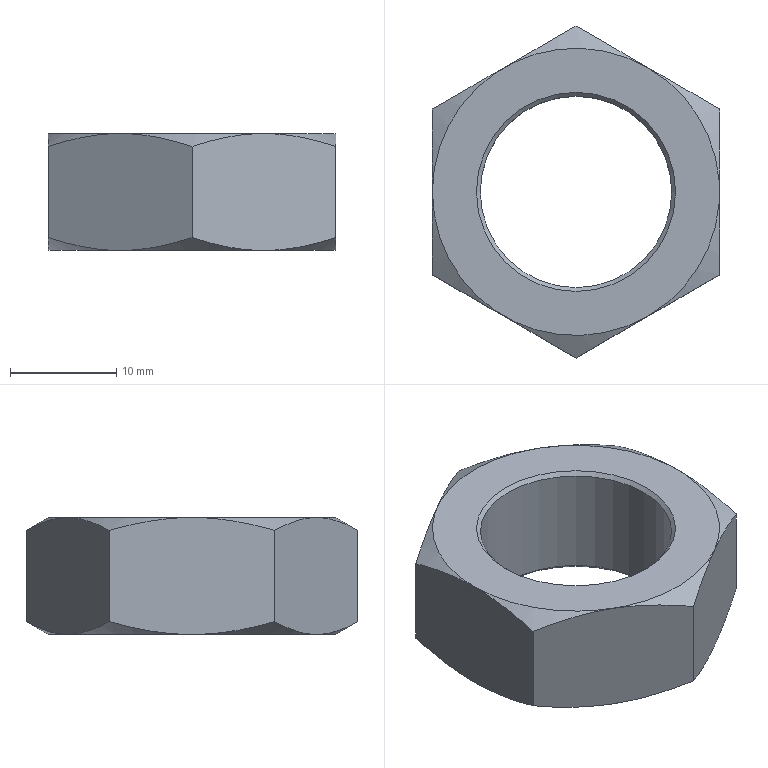Part | NX | features Hydraulic2.3_M18X1.5 2 | 1 solid | 13 faces | box 27.02 x 31.2 x 11 mm | volume 4104 mm3 | plane 8 | cone 4 | cylinder 1 | commonest cylinder face diameters 18 x1
STEP:
#1=CARTESIAN_POINT('',(-13.5,0.,5.5));
#2=VERTEX_POINT('',#1);
#3=CARTESIAN_POINT('',(0.,0.,5.5));
#4=DIRECTION('',(0.,0.,-1.));
#5=DIRECTION('',(-1.,0.,0.));
#6=AXIS2_PLACEMENT_3D('',#3,#4,#5);
#7=CIRCLE('',#6,13.5);
#8=EDGE_CURVE('',#2,#2,#7,.T.);
#9=ORIENTED_EDGE('',*,*,#8,.F.);
#10=EDGE_LOOP('',(#9));
#11=FACE_BOUND('',#10,.T.);
#12=CARTESIAN_POINT('',(9.36,0.,5.5));
#13=VERTEX_POINT('',#12);
#14=CARTESIAN_POINT('',(0.,0.,5.5));
#15=DIRECTION('',(0.,0.,1.));
#16=DIRECTION('',(1.,0.,0.));
#17=AXIS2_PLACEMENT_3D('',#14,#15,#16);
#18=CIRCLE('',#17,9.36);
#19=EDGE_CURVE('',#13,#13,#18,.F.);
#20=ORIENTED_EDGE('',*,*,#19,.T.);
#21=EDGE_LOOP('',(#20));
#22=FACE_BOUND('',#21,.T.);
#23=CARTESIAN_POINT('',(0.,9.,5.5));
#24=DIRECTION('',(0.,0.,1.));
#25=DIRECTION('',(0.,-1.,0.));
#26=AXIS2_PLACEMENT_3D('',#23,#24,#25);
#27=PLANE('',#26);
#28=ADVANCED_FACE('',(#11,#22),#27,.T.);
#29=CARTESIAN_POINT('',(0.,9.,5.14));
#30=VERTEX_POINT('',#29);
#31=CARTESIAN_POINT('',(0.,0.,5.14));
#32=DIRECTION('',(0.,0.,-1.));
#33=DIRECTION('',(0.,1.,0.));
#34=AXIS2_PLACEMENT_3D('',#31,#32,#33);
#35=CIRCLE('',#34,9.);
#36=EDGE_CURVE('',#30,#30,#35,.T.);
#37=ORIENTED_EDGE('',*,*,#36,.T.);
#38=EDGE_LOOP('',(#37));
#39=FACE_BOUND('',#38,.T.);
#40=ORIENTED_EDGE('',*,*,#19,.F.);
#41=EDGE_LOOP('',(#40));
#42=FACE_BOUND('',#41,.T.);
#43=CARTESIAN_POINT('',(0.,0.,5.5));
#44=DIRECTION('',(0.,0.,1.));
#45=DIRECTION('',(1.,0.,0.));
#46=AXIS2_PLACEMENT_3D('',#43,#44,#45);
#47=CONICAL_SURFACE('',#46,9.36,0.7854);
#48=ADVANCED_FACE('',(#39,#42),#47,.F.);
#49=ORIENTED_EDGE('',*,*,#8,.T.);
#50=EDGE_LOOP('',(#49));
#51=FACE_BOUND('',#50,.T.);
#52=CARTESIAN_POINT('',(13.51,-7.8,4.288));
#53=VERTEX_POINT('',#52);
#54=CARTESIAN_POINT('',(0.,-15.6,4.288));
#55=VERTEX_POINT('',#54);
#56=CARTESIAN_POINT('',(13.51,-7.8,4.288));
#57=CARTESIAN_POINT('',(11.304,-9.074,5.023));
#58=CARTESIAN_POINT('',(6.779,-11.686,5.965));
#59=CARTESIAN_POINT('',(2.209,-14.325,5.024));
#60=CARTESIAN_POINT('',(0.,-15.6,4.288));
#61=B_SPLINE_CURVE_WITH_KNOTS('',3,(#56,#57,#58,#59,#60),.UNSPECIFIED.,.F.,.F.,(4,1,4),(0.,0.007878,0.01576),.UNSPECIFIED.);
#62=EDGE_CURVE('',#53,#55,#61,.T.);
#63=ORIENTED_EDGE('',*,*,#62,.F.);
#64=CARTESIAN_POINT('',(13.51,7.8,4.288));
#65=VERTEX_POINT('',#64);
#66=CARTESIAN_POINT('',(13.51,7.8,4.288));
#67=CARTESIAN_POINT('',(13.51,5.252,5.023));
#68=CARTESIAN_POINT('',(13.51,0.,5.965));
#69=CARTESIAN_POINT('',(13.51,-5.252,5.023));
#70=CARTESIAN_POINT('',(13.51,-7.8,4.288));
#71=B_SPLINE_CURVE_WITH_KNOTS('',3,(#66,#67,#68,#69,#70),.UNSPECIFIED.,.F.,.F.,(4,1,4),(-0.007893,0.,0.007893),.UNSPECIFIED.);
#72=EDGE_CURVE('',#65,#53,#71,.T.);
#73=ORIENTED_EDGE('',*,*,#72,.F.);
#74=CARTESIAN_POINT('',(0.,15.6,4.288));
#75=VERTEX_POINT('',#74);
#76=CARTESIAN_POINT('',(0.,15.6,4.288));
#77=CARTESIAN_POINT('',(2.206,14.326,5.023));
#78=CARTESIAN_POINT('',(6.731,11.714,5.965));
#79=CARTESIAN_POINT('',(11.301,9.075,5.024));
#80=CARTESIAN_POINT('',(13.51,7.8,4.288));
#81=B_SPLINE_CURVE_WITH_KNOTS('',3,(#76,#77,#78,#79,#80),.UNSPECIFIED.,.F.,.F.,(4,1,4),(0.,0.007878,0.01576),.UNSPECIFIED.);
#82=EDGE_CURVE('',#75,#65,#81,.T.);
#83=ORIENTED_EDGE('',*,*,#82,.F.);
#84=CARTESIAN_POINT('',(-13.51,7.8,4.288));
#85=VERTEX_POINT('',#84);
#86=CARTESIAN_POINT('',(-13.51,7.8,4.288));
#87=CARTESIAN_POINT('',(-11.304,9.074,5.023));
#88=CARTESIAN_POINT('',(-6.779,11.686,5.965));
#89=CARTESIAN_POINT('',(-2.209,14.325,5.024));
#90=CARTESIAN_POINT('',(0.,15.6,4.288));
#91=B_SPLINE_CURVE_WITH_KNOTS('',3,(#86,#87,#88,#89,#90),.UNSPECIFIED.,.F.,.F.,(4,1,4),(0.,0.007878,0.01576),.UNSPECIFIED.);
#92=EDGE_CURVE('',#85,#75,#91,.T.);
#93=ORIENTED_EDGE('',*,*,#92,.F.);
#94=CARTESIAN_POINT('',(-13.51,-7.8,4.288));
#95=VERTEX_POINT('',#94);
#96=CARTESIAN_POINT('',(-13.51,-7.8,4.288));
#97=CARTESIAN_POINT('',(-13.51,-5.252,5.023));
#98=CARTESIAN_POINT('',(-13.51,0.,5.965));
#99=CARTESIAN_POINT('',(-13.51,5.252,5.023));
#100=CARTESIAN_POINT('',(-13.51,7.8,4.288));
#101=B_SPLINE_CURVE_WITH_KNOTS('',3,(#96,#97,#98,#99,#100),.UNSPECIFIED.,.F.,.F.,(4,1,4),(-0.007893,0.,0.007893),.UNSPECIFIED.);
#102=EDGE_CURVE('',#95,#85,#101,.T.);
#103=ORIENTED_EDGE('',*,*,#102,.F.);
#104=CARTESIAN_POINT('',(0.,-15.6,4.288));
#105=CARTESIAN_POINT('',(-2.206,-14.326,5.023));
#106=CARTESIAN_POINT('',(-6.731,-11.714,5.965));
#107=CARTESIAN_POINT('',(-11.301,-9.075,5.024));
#108=CARTESIAN_POINT('',(-13.51,-7.8,4.288));
#109=B_SPLINE_CURVE_WITH_KNOTS('',3,(#104,#105,#106,#107,#108),.UNSPECIFIED.,.F.,.F.,(4,1,4),(0.,0.007878,0.01576),.UNSPECIFIED.);
#110=EDGE_CURVE('',#55,#95,#109,.T.);
#111=ORIENTED_EDGE('',*,*,#110,.F.);
#112=EDGE_LOOP('',(#63,#73,#83,#93,#103,#111));
#113=FACE_BOUND('',#112,.T.);
#114=CARTESIAN_POINT('',(0.,0.,4.28));
#115=DIRECTION('',(0.,0.,-1.));
#116=DIRECTION('',(-1.,0.,0.));
#117=AXIS2_PLACEMENT_3D('',#114,#115,#116);
#118=CONICAL_SURFACE('',#117,15.613,1.047);
#119=ADVANCED_FACE('',(#51,#113),#118,.T.);
#120=ORIENTED_EDGE('',*,*,#36,.F.);
#121=EDGE_LOOP('',(#120));
#122=FACE_BOUND('',#121,.T.);
#123=CARTESIAN_POINT('',(-9.,0.,-5.14));
#124=VERTEX_POINT('',#123);
#125=CARTESIAN_POINT('',(0.,0.,-5.14));
#126=DIRECTION('',(0.,0.,-1.));
#127=DIRECTION('',(-1.,0.,0.));
#128=AXIS2_PLACEMENT_3D('',#125,#126,#127);
#129=CIRCLE('',#128,9.);
#130=EDGE_CURVE('',#124,#124,#129,.T.);
#131=ORIENTED_EDGE('',*,*,#130,.T.);
#132=EDGE_LOOP('',(#131));
#133=FACE_BOUND('',#132,.T.);
#134=CARTESIAN_POINT('',(0.,0.,27.389));
#135=DIRECTION('',(0.,0.,-1.));
#136=DIRECTION('',(0.,1.,0.));
#137=AXIS2_PLACEMENT_3D('',#134,#135,#136);
#138=CYLINDRICAL_SURFACE('',#137,9.);
#139=ADVANCED_FACE('',(#122,#133),#138,.F.);
#140=CARTESIAN_POINT('',(0.000000014,-15.6,-4.288));
#141=VERTEX_POINT('',#140);
#142=CARTESIAN_POINT('',(0.,-15.6,-5.5));
#143=DIRECTION('',(0.,0.,1.));
#144=VECTOR('',#143,1000.);
#145=LINE('',#142,#144);
#146=EDGE_CURVE('',#141,#55,#145,.T.);
#147=ORIENTED_EDGE('',*,*,#146,.F.);
#148=CARTESIAN_POINT('',(13.51,-7.8,-4.288));
#149=VERTEX_POINT('',#148);
#150=CARTESIAN_POINT('',(13.51,-7.8,-4.288));
#151=CARTESIAN_POINT('',(11.304,-9.074,-5.023));
#152=CARTESIAN_POINT('',(6.779,-11.686,-5.965));
#153=CARTESIAN_POINT('',(2.209,-14.325,-5.024));
#154=CARTESIAN_POINT('',(0.000000075,-15.6,-4.288));
#155=B_SPLINE_CURVE_WITH_KNOTS('',3,(#150,#151,#152,#153,#154),.UNSPECIFIED.,.F.,.F.,(4,1,4),(0.,0.007878,0.01576),.UNSPECIFIED.);
#156=EDGE_CURVE('',#149,#141,#155,.T.);
#157=ORIENTED_EDGE('',*,*,#156,.F.);
#158=CARTESIAN_POINT('',(13.51,-7.8,-5.5));
#159=DIRECTION('',(0.,0.,1.));
#160=VECTOR('',#159,1000.);
#161=LINE('',#158,#160);
#162=EDGE_CURVE('',#53,#149,#161,.F.);
#163=ORIENTED_EDGE('',*,*,#162,.F.);
#164=ORIENTED_EDGE('',*,*,#62,.T.);
#165=EDGE_LOOP('',(#147,#157,#163,#164));
#166=FACE_BOUND('',#165,.T.);
#167=CARTESIAN_POINT('',(0.,-15.6,-5.5));
#168=DIRECTION('',(0.5,-0.866,0.));
#169=DIRECTION('',(0.866,0.5,0.));
#170=AXIS2_PLACEMENT_3D('',#167,#168,#169);
#171=PLANE('',#170);
#172=ADVANCED_FACE('',(#166),#171,.T.);
#173=CARTESIAN_POINT('',(-13.51,-7.8,-4.288));
#174=VERTEX_POINT('',#173);
#175=CARTESIAN_POINT('',(-13.51,-7.8,-5.5));
#176=DIRECTION('',(0.,0.,1.));
#177=VECTOR('',#176,1000.);
#178=LINE('',#175,#177);
#179=EDGE_CURVE('',#174,#95,#178,.T.);
#180=ORIENTED_EDGE('',*,*,#179,.F.);
#181=CARTESIAN_POINT('',(0.000000042,-15.6,-4.288));
#182=CARTESIAN_POINT('',(-2.206,-14.326,-5.023));
#183=CARTESIAN_POINT('',(-6.731,-11.714,-5.965));
#184=CARTESIAN_POINT('',(-11.301,-9.075,-5.024));
#185=CARTESIAN_POINT('',(-13.51,-7.8,-4.288));
#186=B_SPLINE_CURVE_WITH_KNOTS('',3,(#181,#182,#183,#184,#185),.UNSPECIFIED.,.F.,.F.,(4,1,4),(0.,0.007878,0.01576),.UNSPECIFIED.);
#187=EDGE_CURVE('',#141,#174,#186,.T.);
#188=ORIENTED_EDGE('',*,*,#187,.F.);
#189=ORIENTED_EDGE('',*,*,#146,.T.);
#190=ORIENTED_EDGE('',*,*,#110,.T.);
#191=EDGE_LOOP('',(#180,#188,#189,#190));
#192=FACE_BOUND('',#191,.T.);
#193=CARTESIAN_POINT('',(-13.51,-7.8,-5.5));
#194=DIRECTION('',(-0.5,-0.866,0.));
#195=DIRECTION('',(0.866,-0.5,0.));
#196=AXIS2_PLACEMENT_3D('',#193,#194,#195);
#197=PLANE('',#196);
#198=ADVANCED_FACE('',(#192),#197,.T.);
#199=CARTESIAN_POINT('',(-13.51,7.8,-4.288));
#200=VERTEX_POINT('',#199);
#201=CARTESIAN_POINT('',(-13.51,-7.8,-4.288));
#202=CARTESIAN_POINT('',(-13.51,-5.252,-5.023));
#203=CARTESIAN_POINT('',(-13.51,0.000000059,-5.965));
#204=CARTESIAN_POINT('',(-13.51,5.252,-5.023));
#205=CARTESIAN_POINT('',(-13.51,7.8,-4.288));
#206=B_SPLINE_CURVE_WITH_KNOTS('',3,(#201,#202,#203,#204,#205),.UNSPECIFIED.,.F.,.F.,(4,1,4),(-0.007893,0.,0.007893),.UNSPECIFIED.);
#207=EDGE_CURVE('',#174,#200,#206,.T.);
#208=ORIENTED_EDGE('',*,*,#207,.F.);
#209=ORIENTED_EDGE('',*,*,#179,.T.);
#210=ORIENTED_EDGE('',*,*,#102,.T.);
#211=CARTESIAN_POINT('',(-13.51,7.8,-5.5));
#212=DIRECTION('',(0.,0.,1.));
#213=VECTOR('',#212,1000.);
#214=LINE('',#211,#213);
#215=EDGE_CURVE('',#200,#85,#214,.T.);
#216=ORIENTED_EDGE('',*,*,#215,.F.);
#217=EDGE_LOOP('',(#208,#209,#210,#216));
#218=FACE_BOUND('',#217,.T.);
#219=CARTESIAN_POINT('',(-13.51,7.8,-5.5));
#220=DIRECTION('',(-1.,0.,0.));
#221=DIRECTION('',(0.,-1.,0.));
#222=AXIS2_PLACEMENT_3D('',#219,#220,#221);
#223=PLANE('',#222);
#224=ADVANCED_FACE('',(#218),#223,.T.);
#225=CARTESIAN_POINT('',(-0.000000014,15.6,-4.288));
#226=VERTEX_POINT('',#225);
#227=CARTESIAN_POINT('',(0.,15.6,-5.5));
#228=DIRECTION('',(0.,0.,1.));
#229=VECTOR('',#228,1000.);
#230=LINE('',#227,#229);
#231=EDGE_CURVE('',#226,#75,#230,.T.);
#232=ORIENTED_EDGE('',*,*,#231,.F.);
#233=CARTESIAN_POINT('',(-13.51,7.8,-4.288));
#234=CARTESIAN_POINT('',(-11.304,9.074,-5.023));
#235=CARTESIAN_POINT('',(-6.779,11.686,-5.965));
#236=CARTESIAN_POINT('',(-2.209,14.325,-5.024));
#237=CARTESIAN_POINT('',(-0.000000075,15.6,-4.288));
#238=B_SPLINE_CURVE_WITH_KNOTS('',3,(#233,#234,#235,#236,#237),.UNSPECIFIED.,.F.,.F.,(4,1,4),(0.,0.007878,0.01576),.UNSPECIFIED.);
#239=EDGE_CURVE('',#200,#226,#238,.T.);
#240=ORIENTED_EDGE('',*,*,#239,.F.);
#241=ORIENTED_EDGE('',*,*,#215,.T.);
#242=ORIENTED_EDGE('',*,*,#92,.T.);
#243=EDGE_LOOP('',(#232,#240,#241,#242));
#244=FACE_BOUND('',#243,.T.);
#245=CARTESIAN_POINT('',(0.,15.6,-5.5));
#246=DIRECTION('',(-0.5,0.866,0.));
#247=DIRECTION('',(-0.866,-0.5,0.));
#248=AXIS2_PLACEMENT_3D('',#245,#246,#247);
#249=PLANE('',#248);
#250=ADVANCED_FACE('',(#244),#249,.T.);
#251=CARTESIAN_POINT('',(13.51,7.8,-4.288));
#252=VERTEX_POINT('',#251);
#253=CARTESIAN_POINT('',(13.51,7.8,-5.5));
#254=DIRECTION('',(0.,0.,1.));
#255=VECTOR('',#254,1000.);
#256=LINE('',#253,#255);
#257=EDGE_CURVE('',#252,#65,#256,.T.);
#258=ORIENTED_EDGE('',*,*,#257,.F.);
#259=CARTESIAN_POINT('',(-0.000000029,15.6,-4.288));
#260=CARTESIAN_POINT('',(2.206,14.326,-5.023));
#261=CARTESIAN_POINT('',(6.731,11.714,-5.965));
#262=CARTESIAN_POINT('',(11.301,9.075,-5.024));
#263=CARTESIAN_POINT('',(13.51,7.8,-4.288));
#264=B_SPLINE_CURVE_WITH_KNOTS('',3,(#259,#260,#261,#262,#263),.UNSPECIFIED.,.F.,.F.,(4,1,4),(0.,0.007878,0.01576),.UNSPECIFIED.);
#265=EDGE_CURVE('',#226,#252,#264,.T.);
#266=ORIENTED_EDGE('',*,*,#265,.F.);
#267=ORIENTED_EDGE('',*,*,#231,.T.);
#268=ORIENTED_EDGE('',*,*,#82,.T.);
#269=EDGE_LOOP('',(#258,#266,#267,#268));
#270=FACE_BOUND('',#269,.T.);
#271=CARTESIAN_POINT('',(13.51,7.8,-5.5));
#272=DIRECTION('',(0.5,0.866,0.));
#273=DIRECTION('',(-0.866,0.5,0.));
#274=AXIS2_PLACEMENT_3D('',#271,#272,#273);
#275=PLANE('',#274);
#276=ADVANCED_FACE('',(#270),#275,.T.);
#277=ORIENTED_EDGE('',*,*,#162,.T.);
#278=CARTESIAN_POINT('',(13.51,7.8,-4.288));
#279=CARTESIAN_POINT('',(13.51,5.252,-5.023));
#280=CARTESIAN_POINT('',(13.51,-0.000000059,-5.965));
#281=CARTESIAN_POINT('',(13.51,-5.252,-5.023));
#282=CARTESIAN_POINT('',(13.51,-7.8,-4.288));
#283=B_SPLINE_CURVE_WITH_KNOTS('',3,(#278,#279,#280,#281,#282),.UNSPECIFIED.,.F.,.F.,(4,1,4),(0.,0.007893,0.01579),.UNSPECIFIED.);
#284=EDGE_CURVE('',#252,#149,#283,.T.);
#285=ORIENTED_EDGE('',*,*,#284,.F.);
#286=ORIENTED_EDGE('',*,*,#257,.T.);
#287=ORIENTED_EDGE('',*,*,#72,.T.);
#288=EDGE_LOOP('',(#277,#285,#286,#287));
#289=FACE_BOUND('',#288,.T.);
#290=CARTESIAN_POINT('',(13.51,-7.8,-5.5));
#291=DIRECTION('',(1.,0.,0.));
#292=DIRECTION('',(0.,1.,0.));
#293=AXIS2_PLACEMENT_3D('',#290,#291,#292);
#294=PLANE('',#293);
#295=ADVANCED_FACE('',(#289),#294,.T.);
#296=ORIENTED_EDGE('',*,*,#130,.F.);
#297=EDGE_LOOP('',(#296));
#298=FACE_BOUND('',#297,.T.);
#299=CARTESIAN_POINT('',(-9.36,0.,-5.5));
#300=VERTEX_POINT('',#299);
#301=CARTESIAN_POINT('',(0.,0.,-5.5));
#302=DIRECTION('',(0.,0.,-1.));
#303=DIRECTION('',(-1.,0.,0.));
#304=AXIS2_PLACEMENT_3D('',#301,#302,#303);
#305=CIRCLE('',#304,9.36);
#306=EDGE_CURVE('',#300,#300,#305,.F.);
#307=ORIENTED_EDGE('',*,*,#306,.F.);
#308=EDGE_LOOP('',(#307));
#309=FACE_BOUND('',#308,.T.);
#310=CARTESIAN_POINT('',(0.,0.,-5.5));
#311=DIRECTION('',(0.,0.,-1.));
#312=DIRECTION('',(-1.,0.,0.));
#313=AXIS2_PLACEMENT_3D('',#310,#311,#312);
#314=CONICAL_SURFACE('',#313,9.36,0.7854);
#315=ADVANCED_FACE('',(#298,#309),#314,.F.);
#316=ORIENTED_EDGE('',*,*,#187,.T.);
#317=ORIENTED_EDGE('',*,*,#207,.T.);
#318=ORIENTED_EDGE('',*,*,#239,.T.);
#319=ORIENTED_EDGE('',*,*,#265,.T.);
#320=ORIENTED_EDGE('',*,*,#284,.T.);
#321=ORIENTED_EDGE('',*,*,#156,.T.);
#322=EDGE_LOOP('',(#316,#317,#318,#319,#320,#321));
#323=FACE_BOUND('',#322,.T.);
#324=CARTESIAN_POINT('',(13.5,0.,-5.5));
#325=VERTEX_POINT('',#324);
#326=CARTESIAN_POINT('',(0.,0.,-5.5));
#327=DIRECTION('',(0.,0.,1.));
#328=DIRECTION('',(1.,0.,0.));
#329=AXIS2_PLACEMENT_3D('',#326,#327,#328);
#330=CIRCLE('',#329,13.5);
#331=EDGE_CURVE('',#325,#325,#330,.F.);
#332=ORIENTED_EDGE('',*,*,#331,.F.);
#333=EDGE_LOOP('',(#332));
#334=FACE_BOUND('',#333,.T.);
#335=CARTESIAN_POINT('',(0.,0.,-4.28));
#336=DIRECTION('',(0.,0.,1.));
#337=DIRECTION('',(1.,0.,0.));
#338=AXIS2_PLACEMENT_3D('',#335,#336,#337);
#339=CONICAL_SURFACE('',#338,15.613,1.047);
#340=ADVANCED_FACE('',(#323,#334),#339,.T.);
#341=ORIENTED_EDGE('',*,*,#331,.T.);
#342=EDGE_LOOP('',(#341));
#343=FACE_BOUND('',#342,.T.);
#344=ORIENTED_EDGE('',*,*,#306,.T.);
#345=EDGE_LOOP('',(#344));
#346=FACE_BOUND('',#345,.T.);
#347=CARTESIAN_POINT('',(0.,9.,-5.5));
#348=DIRECTION('',(0.,0.,-1.));
#349=DIRECTION('',(0.,1.,0.));
#350=AXIS2_PLACEMENT_3D('',#347,#348,#349);
#351=PLANE('',#350);
#352=ADVANCED_FACE('',(#343,#346),#351,.T.);
#353=CLOSED_SHELL('',(#28,#48,#119,#139,#172,#198,#224,#250,#276,#295,#315,#340,#352));
#354=MANIFOLD_SOLID_BREP('',#353);
#355=(LENGTH_UNIT()NAMED_UNIT(*)SI_UNIT(.MILLI.,.METRE.));
#356=UNCERTAINTY_MEASURE_WITH_UNIT(LENGTH_MEASURE(0.0508),#355,'','');
#357=(NAMED_UNIT(*)PLANE_ANGLE_UNIT()SI_UNIT($,.RADIAN.));
#358=(NAMED_UNIT(*)SI_UNIT($,.STERADIAN.)SOLID_ANGLE_UNIT());
#359=(GEOMETRIC_REPRESENTATION_CONTEXT(3)GLOBAL_UNCERTAINTY_ASSIGNED_CONTEXT((#356))GLOBAL_UNIT_ASSIGNED_CONTEXT((#355,#357,#358))REPRESENTATION_CONTEXT('',''));
#360=ADVANCED_BREP_SHAPE_REPRESENTATION('',(#354),#359);